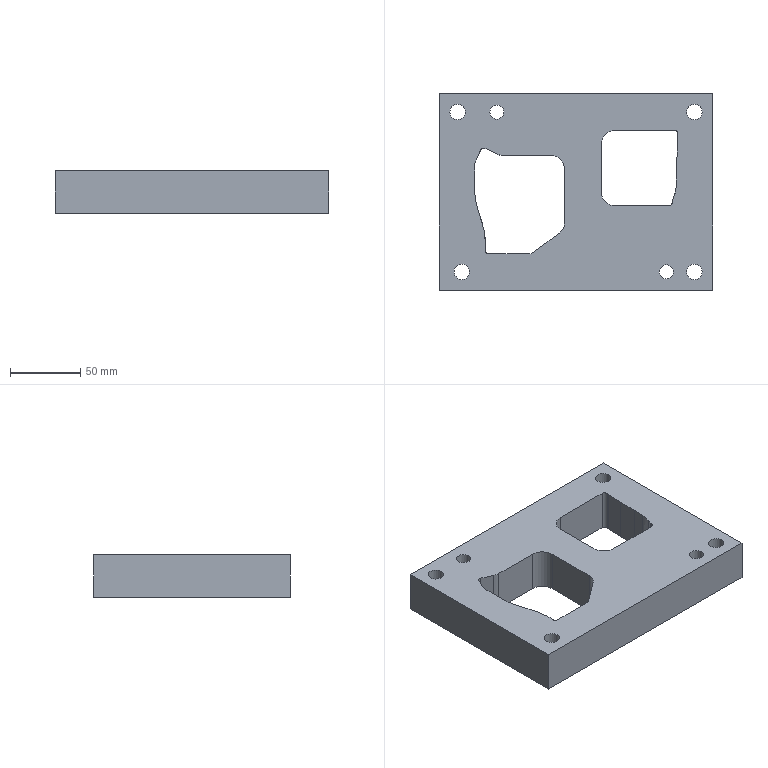Part | STEP file | 207_id706_x_t | 1 solid | 56 faces | box 195 x 140 x 30 mm | volume 585994 mm3 | cylinder 26 | plane 23 | other 7 | commonest cylinder face diameters 5 x8 11 x6 20 x5 17 x4 10 x3